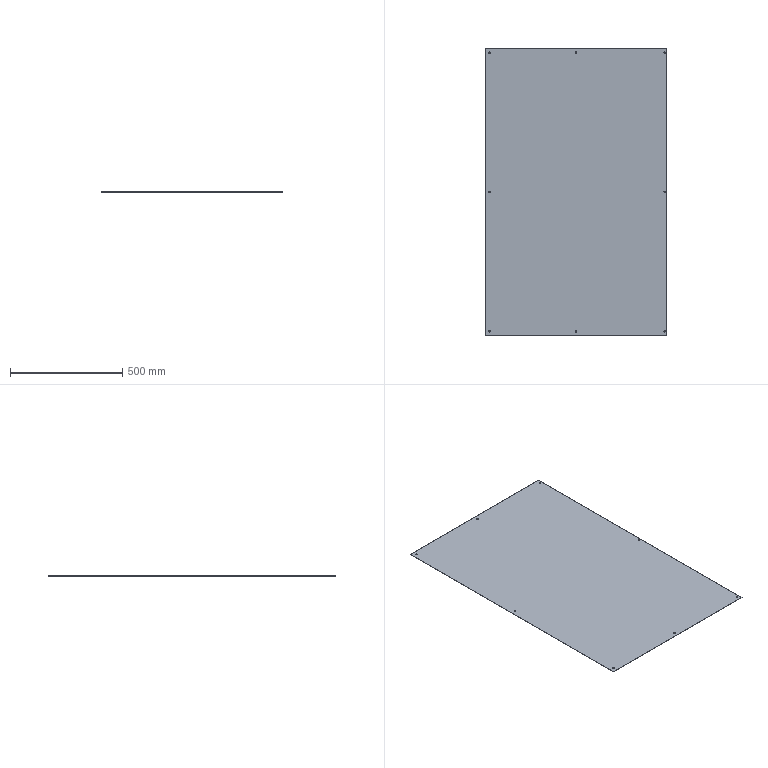Part | SolidWorks | features FlatPattern 1, HoleWzd 1, SMBaseFlange 1, SheetMetal 1 | 1 solid | 22 faces | box 810 x 1280 x 1.2 mm | volume 1243832 mm3 | cylinder 16 | plane 6 | commonest cylinder face diameters 6.6 x16
STEP:
#1=CARTESIAN_POINT('',(-388.3,620.,-1.2));
#2=VERTEX_POINT('',#1);
#3=CARTESIAN_POINT('',(-381.7,620.,-1.2));
#4=VERTEX_POINT('',#3);
#5=CARTESIAN_POINT('',(-385.,620.,-1.2));
#6=DIRECTION('',(0.,0.,1.));
#7=DIRECTION('',(1.,0.,0.));
#8=AXIS2_PLACEMENT_3D('',#5,#6,#7);
#9=CIRCLE('',#8,3.3);
#10=EDGE_CURVE('',#2,#4,#9,.T.);
#11=ORIENTED_EDGE('',*,*,#10,.F.);
#12=CARTESIAN_POINT('',(-388.3,620.,0.));
#13=VERTEX_POINT('',#12);
#14=CARTESIAN_POINT('',(-388.3,620.,0.));
#15=DIRECTION('',(0.,0.,1.));
#16=VECTOR('',#15,1000.);
#17=LINE('',#14,#16);
#18=EDGE_CURVE('',#2,#13,#17,.T.);
#19=ORIENTED_EDGE('',*,*,#18,.T.);
#20=CARTESIAN_POINT('',(-381.7,620.,0.));
#21=VERTEX_POINT('',#20);
#22=CARTESIAN_POINT('',(-385.,620.,0.));
#23=DIRECTION('',(0.,0.,1.));
#24=DIRECTION('',(1.,0.,0.));
#25=AXIS2_PLACEMENT_3D('',#22,#23,#24);
#26=CIRCLE('',#25,3.3);
#27=EDGE_CURVE('',#13,#21,#26,.T.);
#28=ORIENTED_EDGE('',*,*,#27,.T.);
#29=CARTESIAN_POINT('',(-381.7,620.,0.));
#30=DIRECTION('',(0.,0.,1.));
#31=VECTOR('',#30,1000.);
#32=LINE('',#29,#31);
#33=EDGE_CURVE('',#4,#21,#32,.T.);
#34=ORIENTED_EDGE('',*,*,#33,.F.);
#35=EDGE_LOOP('',(#11,#19,#28,#34));
#36=FACE_OUTER_BOUND('',#35,.T.);
#37=CARTESIAN_POINT('',(-385.,620.,0.));
#38=DIRECTION('',(0.,0.,1.));
#39=DIRECTION('',(1.,0.,0.));
#40=AXIS2_PLACEMENT_3D('',#37,#38,#39);
#41=CYLINDRICAL_SURFACE('',#40,3.3);
#42=ADVANCED_FACE('',(#36),#41,.F.);
#43=CARTESIAN_POINT('',(-3.3,620.,-1.2));
#44=VERTEX_POINT('',#43);
#45=CARTESIAN_POINT('',(3.3,620.,-1.2));
#46=VERTEX_POINT('',#45);
#47=CARTESIAN_POINT('',(0.,620.,-1.2));
#48=DIRECTION('',(0.,0.,1.));
#49=DIRECTION('',(1.,0.,0.));
#50=AXIS2_PLACEMENT_3D('',#47,#48,#49);
#51=CIRCLE('',#50,3.3);
#52=EDGE_CURVE('',#44,#46,#51,.T.);
#53=ORIENTED_EDGE('',*,*,#52,.F.);
#54=CARTESIAN_POINT('',(-3.3,620.,0.));
#55=VERTEX_POINT('',#54);
#56=CARTESIAN_POINT('',(-3.3,620.,0.));
#57=DIRECTION('',(0.,0.,1.));
#58=VECTOR('',#57,1000.);
#59=LINE('',#56,#58);
#60=EDGE_CURVE('',#44,#55,#59,.T.);
#61=ORIENTED_EDGE('',*,*,#60,.T.);
#62=CARTESIAN_POINT('',(3.3,620.,0.));
#63=VERTEX_POINT('',#62);
#64=CARTESIAN_POINT('',(0.,620.,0.));
#65=DIRECTION('',(0.,0.,1.));
#66=DIRECTION('',(1.,0.,0.));
#67=AXIS2_PLACEMENT_3D('',#64,#65,#66);
#68=CIRCLE('',#67,3.3);
#69=EDGE_CURVE('',#55,#63,#68,.T.);
#70=ORIENTED_EDGE('',*,*,#69,.T.);
#71=CARTESIAN_POINT('',(3.3,620.,0.));
#72=DIRECTION('',(0.,0.,1.));
#73=VECTOR('',#72,1000.);
#74=LINE('',#71,#73);
#75=EDGE_CURVE('',#46,#63,#74,.T.);
#76=ORIENTED_EDGE('',*,*,#75,.F.);
#77=EDGE_LOOP('',(#53,#61,#70,#76));
#78=FACE_OUTER_BOUND('',#77,.T.);
#79=CARTESIAN_POINT('',(0.,620.,0.));
#80=DIRECTION('',(0.,0.,1.));
#81=DIRECTION('',(1.,0.,0.));
#82=AXIS2_PLACEMENT_3D('',#79,#80,#81);
#83=CYLINDRICAL_SURFACE('',#82,3.3);
#84=ADVANCED_FACE('',(#78),#83,.F.);
#85=CARTESIAN_POINT('',(391.7,620.,-1.2));
#86=VERTEX_POINT('',#85);
#87=CARTESIAN_POINT('',(398.3,620.,-1.2));
#88=VERTEX_POINT('',#87);
#89=CARTESIAN_POINT('',(395.,620.,-1.2));
#90=DIRECTION('',(0.,0.,1.));
#91=DIRECTION('',(1.,0.,0.));
#92=AXIS2_PLACEMENT_3D('',#89,#90,#91);
#93=CIRCLE('',#92,3.3);
#94=EDGE_CURVE('',#86,#88,#93,.T.);
#95=ORIENTED_EDGE('',*,*,#94,.F.);
#96=CARTESIAN_POINT('',(391.7,620.,0.));
#97=VERTEX_POINT('',#96);
#98=CARTESIAN_POINT('',(391.7,620.,0.));
#99=DIRECTION('',(0.,0.,1.));
#100=VECTOR('',#99,1000.);
#101=LINE('',#98,#100);
#102=EDGE_CURVE('',#86,#97,#101,.T.);
#103=ORIENTED_EDGE('',*,*,#102,.T.);
#104=CARTESIAN_POINT('',(398.3,620.,0.));
#105=VERTEX_POINT('',#104);
#106=CARTESIAN_POINT('',(395.,620.,0.));
#107=DIRECTION('',(0.,0.,1.));
#108=DIRECTION('',(1.,0.,0.));
#109=AXIS2_PLACEMENT_3D('',#106,#107,#108);
#110=CIRCLE('',#109,3.3);
#111=EDGE_CURVE('',#97,#105,#110,.T.);
#112=ORIENTED_EDGE('',*,*,#111,.T.);
#113=CARTESIAN_POINT('',(398.3,620.,0.));
#114=DIRECTION('',(0.,0.,1.));
#115=VECTOR('',#114,1000.);
#116=LINE('',#113,#115);
#117=EDGE_CURVE('',#88,#105,#116,.T.);
#118=ORIENTED_EDGE('',*,*,#117,.F.);
#119=EDGE_LOOP('',(#95,#103,#112,#118));
#120=FACE_OUTER_BOUND('',#119,.T.);
#121=CARTESIAN_POINT('',(395.,620.,0.));
#122=DIRECTION('',(0.,0.,1.));
#123=DIRECTION('',(1.,0.,0.));
#124=AXIS2_PLACEMENT_3D('',#121,#122,#123);
#125=CYLINDRICAL_SURFACE('',#124,3.3);
#126=ADVANCED_FACE('',(#120),#125,.F.);
#127=CARTESIAN_POINT('',(391.7,0.,-1.2));
#128=VERTEX_POINT('',#127);
#129=CARTESIAN_POINT('',(398.3,0.,-1.2));
#130=VERTEX_POINT('',#129);
#131=CARTESIAN_POINT('',(395.,0.,-1.2));
#132=DIRECTION('',(0.,0.,1.));
#133=DIRECTION('',(1.,0.,0.));
#134=AXIS2_PLACEMENT_3D('',#131,#132,#133);
#135=CIRCLE('',#134,3.3);
#136=EDGE_CURVE('',#128,#130,#135,.T.);
#137=ORIENTED_EDGE('',*,*,#136,.F.);
#138=CARTESIAN_POINT('',(391.7,0.,0.));
#139=VERTEX_POINT('',#138);
#140=CARTESIAN_POINT('',(391.7,0.,0.));
#141=DIRECTION('',(0.,0.,1.));
#142=VECTOR('',#141,1000.);
#143=LINE('',#140,#142);
#144=EDGE_CURVE('',#128,#139,#143,.T.);
#145=ORIENTED_EDGE('',*,*,#144,.T.);
#146=CARTESIAN_POINT('',(398.3,0.,0.));
#147=VERTEX_POINT('',#146);
#148=CARTESIAN_POINT('',(395.,0.,0.));
#149=DIRECTION('',(0.,0.,1.));
#150=DIRECTION('',(1.,0.,0.));
#151=AXIS2_PLACEMENT_3D('',#148,#149,#150);
#152=CIRCLE('',#151,3.3);
#153=EDGE_CURVE('',#139,#147,#152,.T.);
#154=ORIENTED_EDGE('',*,*,#153,.T.);
#155=CARTESIAN_POINT('',(398.3,0.,0.));
#156=DIRECTION('',(0.,0.,1.));
#157=VECTOR('',#156,1000.);
#158=LINE('',#155,#157);
#159=EDGE_CURVE('',#130,#147,#158,.T.);
#160=ORIENTED_EDGE('',*,*,#159,.F.);
#161=EDGE_LOOP('',(#137,#145,#154,#160));
#162=FACE_OUTER_BOUND('',#161,.T.);
#163=CARTESIAN_POINT('',(395.,0.,0.));
#164=DIRECTION('',(0.,0.,1.));
#165=DIRECTION('',(1.,0.,0.));
#166=AXIS2_PLACEMENT_3D('',#163,#164,#165);
#167=CYLINDRICAL_SURFACE('',#166,3.3);
#168=ADVANCED_FACE('',(#162),#167,.F.);
#169=CARTESIAN_POINT('',(391.7,-620.,-1.2));
#170=VERTEX_POINT('',#169);
#171=CARTESIAN_POINT('',(398.3,-620.,-1.2));
#172=VERTEX_POINT('',#171);
#173=CARTESIAN_POINT('',(395.,-620.,-1.2));
#174=DIRECTION('',(0.,0.,1.));
#175=DIRECTION('',(1.,0.,0.));
#176=AXIS2_PLACEMENT_3D('',#173,#174,#175);
#177=CIRCLE('',#176,3.3);
#178=EDGE_CURVE('',#170,#172,#177,.T.);
#179=ORIENTED_EDGE('',*,*,#178,.F.);
#180=CARTESIAN_POINT('',(391.7,-620.,0.));
#181=VERTEX_POINT('',#180);
#182=CARTESIAN_POINT('',(391.7,-620.,0.));
#183=DIRECTION('',(0.,0.,1.));
#184=VECTOR('',#183,1000.);
#185=LINE('',#182,#184);
#186=EDGE_CURVE('',#170,#181,#185,.T.);
#187=ORIENTED_EDGE('',*,*,#186,.T.);
#188=CARTESIAN_POINT('',(398.3,-620.,0.));
#189=VERTEX_POINT('',#188);
#190=CARTESIAN_POINT('',(395.,-620.,0.));
#191=DIRECTION('',(0.,0.,1.));
#192=DIRECTION('',(1.,0.,0.));
#193=AXIS2_PLACEMENT_3D('',#190,#191,#192);
#194=CIRCLE('',#193,3.3);
#195=EDGE_CURVE('',#181,#189,#194,.T.);
#196=ORIENTED_EDGE('',*,*,#195,.T.);
#197=CARTESIAN_POINT('',(398.3,-620.,0.));
#198=DIRECTION('',(0.,0.,1.));
#199=VECTOR('',#198,1000.);
#200=LINE('',#197,#199);
#201=EDGE_CURVE('',#172,#189,#200,.T.);
#202=ORIENTED_EDGE('',*,*,#201,.F.);
#203=EDGE_LOOP('',(#179,#187,#196,#202));
#204=FACE_OUTER_BOUND('',#203,.T.);
#205=CARTESIAN_POINT('',(395.,-620.,0.));
#206=DIRECTION('',(0.,0.,1.));
#207=DIRECTION('',(1.,0.,0.));
#208=AXIS2_PLACEMENT_3D('',#205,#206,#207);
#209=CYLINDRICAL_SURFACE('',#208,3.3);
#210=ADVANCED_FACE('',(#204),#209,.F.);
#211=CARTESIAN_POINT('',(-3.3,-620.,-1.2));
#212=VERTEX_POINT('',#211);
#213=CARTESIAN_POINT('',(3.3,-620.,-1.2));
#214=VERTEX_POINT('',#213);
#215=CARTESIAN_POINT('',(0.,-620.,-1.2));
#216=DIRECTION('',(0.,0.,1.));
#217=DIRECTION('',(1.,0.,0.));
#218=AXIS2_PLACEMENT_3D('',#215,#216,#217);
#219=CIRCLE('',#218,3.3);
#220=EDGE_CURVE('',#212,#214,#219,.T.);
#221=ORIENTED_EDGE('',*,*,#220,.F.);
#222=CARTESIAN_POINT('',(-3.3,-620.,0.));
#223=VERTEX_POINT('',#222);
#224=CARTESIAN_POINT('',(-3.3,-620.,0.));
#225=DIRECTION('',(0.,0.,1.));
#226=VECTOR('',#225,1000.);
#227=LINE('',#224,#226);
#228=EDGE_CURVE('',#212,#223,#227,.T.);
#229=ORIENTED_EDGE('',*,*,#228,.T.);
#230=CARTESIAN_POINT('',(3.3,-620.,0.));
#231=VERTEX_POINT('',#230);
#232=CARTESIAN_POINT('',(0.,-620.,0.));
#233=DIRECTION('',(0.,0.,1.));
#234=DIRECTION('',(1.,0.,0.));
#235=AXIS2_PLACEMENT_3D('',#232,#233,#234);
#236=CIRCLE('',#235,3.3);
#237=EDGE_CURVE('',#223,#231,#236,.T.);
#238=ORIENTED_EDGE('',*,*,#237,.T.);
#239=CARTESIAN_POINT('',(3.3,-620.,0.));
#240=DIRECTION('',(0.,0.,1.));
#241=VECTOR('',#240,1000.);
#242=LINE('',#239,#241);
#243=EDGE_CURVE('',#214,#231,#242,.T.);
#244=ORIENTED_EDGE('',*,*,#243,.F.);
#245=EDGE_LOOP('',(#221,#229,#238,#244));
#246=FACE_OUTER_BOUND('',#245,.T.);
#247=CARTESIAN_POINT('',(0.,-620.,0.));
#248=DIRECTION('',(0.,0.,1.));
#249=DIRECTION('',(1.,0.,0.));
#250=AXIS2_PLACEMENT_3D('',#247,#248,#249);
#251=CYLINDRICAL_SURFACE('',#250,3.3);
#252=ADVANCED_FACE('',(#246),#251,.F.);
#253=CARTESIAN_POINT('',(-388.3,-620.,-1.2));
#254=VERTEX_POINT('',#253);
#255=CARTESIAN_POINT('',(-381.7,-620.,-1.2));
#256=VERTEX_POINT('',#255);
#257=CARTESIAN_POINT('',(-385.,-620.,-1.2));
#258=DIRECTION('',(0.,0.,1.));
#259=DIRECTION('',(1.,0.,0.));
#260=AXIS2_PLACEMENT_3D('',#257,#258,#259);
#261=CIRCLE('',#260,3.3);
#262=EDGE_CURVE('',#254,#256,#261,.T.);
#263=ORIENTED_EDGE('',*,*,#262,.F.);
#264=CARTESIAN_POINT('',(-388.3,-620.,0.));
#265=VERTEX_POINT('',#264);
#266=CARTESIAN_POINT('',(-388.3,-620.,0.));
#267=DIRECTION('',(0.,0.,1.));
#268=VECTOR('',#267,1000.);
#269=LINE('',#266,#268);
#270=EDGE_CURVE('',#254,#265,#269,.T.);
#271=ORIENTED_EDGE('',*,*,#270,.T.);
#272=CARTESIAN_POINT('',(-381.7,-620.,0.));
#273=VERTEX_POINT('',#272);
#274=CARTESIAN_POINT('',(-385.,-620.,0.));
#275=DIRECTION('',(0.,0.,1.));
#276=DIRECTION('',(1.,0.,0.));
#277=AXIS2_PLACEMENT_3D('',#274,#275,#276);
#278=CIRCLE('',#277,3.3);
#279=EDGE_CURVE('',#265,#273,#278,.T.);
#280=ORIENTED_EDGE('',*,*,#279,.T.);
#281=CARTESIAN_POINT('',(-381.7,-620.,0.));
#282=DIRECTION('',(0.,0.,1.));
#283=VECTOR('',#282,1000.);
#284=LINE('',#281,#283);
#285=EDGE_CURVE('',#256,#273,#284,.T.);
#286=ORIENTED_EDGE('',*,*,#285,.F.);
#287=EDGE_LOOP('',(#263,#271,#280,#286));
#288=FACE_OUTER_BOUND('',#287,.T.);
#289=CARTESIAN_POINT('',(-385.,-620.,0.));
#290=DIRECTION('',(0.,0.,1.));
#291=DIRECTION('',(1.,0.,0.));
#292=AXIS2_PLACEMENT_3D('',#289,#290,#291);
#293=CYLINDRICAL_SURFACE('',#292,3.3);
#294=ADVANCED_FACE('',(#288),#293,.F.);
#295=CARTESIAN_POINT('',(-388.3,0.,-1.2));
#296=VERTEX_POINT('',#295);
#297=CARTESIAN_POINT('',(-381.7,0.,-1.2));
#298=VERTEX_POINT('',#297);
#299=CARTESIAN_POINT('',(-385.,0.,-1.2));
#300=DIRECTION('',(0.,0.,1.));
#301=DIRECTION('',(1.,0.,0.));
#302=AXIS2_PLACEMENT_3D('',#299,#300,#301);
#303=CIRCLE('',#302,3.3);
#304=EDGE_CURVE('',#296,#298,#303,.T.);
#305=ORIENTED_EDGE('',*,*,#304,.F.);
#306=CARTESIAN_POINT('',(-388.3,0.,0.));
#307=VERTEX_POINT('',#306);
#308=CARTESIAN_POINT('',(-388.3,0.,0.));
#309=DIRECTION('',(0.,0.,1.));
#310=VECTOR('',#309,1000.);
#311=LINE('',#308,#310);
#312=EDGE_CURVE('',#296,#307,#311,.T.);
#313=ORIENTED_EDGE('',*,*,#312,.T.);
#314=CARTESIAN_POINT('',(-381.7,0.,0.));
#315=VERTEX_POINT('',#314);
#316=CARTESIAN_POINT('',(-385.,0.,0.));
#317=DIRECTION('',(0.,0.,1.));
#318=DIRECTION('',(1.,0.,0.));
#319=AXIS2_PLACEMENT_3D('',#316,#317,#318);
#320=CIRCLE('',#319,3.3);
#321=EDGE_CURVE('',#307,#315,#320,.T.);
#322=ORIENTED_EDGE('',*,*,#321,.T.);
#323=CARTESIAN_POINT('',(-381.7,0.,0.));
#324=DIRECTION('',(0.,0.,1.));
#325=VECTOR('',#324,1000.);
#326=LINE('',#323,#325);
#327=EDGE_CURVE('',#298,#315,#326,.T.);
#328=ORIENTED_EDGE('',*,*,#327,.F.);
#329=EDGE_LOOP('',(#305,#313,#322,#328));
#330=FACE_OUTER_BOUND('',#329,.T.);
#331=CARTESIAN_POINT('',(-385.,0.,0.));
#332=DIRECTION('',(0.,0.,1.));
#333=DIRECTION('',(1.,0.,0.));
#334=AXIS2_PLACEMENT_3D('',#331,#332,#333);
#335=CYLINDRICAL_SURFACE('',#334,3.3);
#336=ADVANCED_FACE('',(#330),#335,.F.);
#337=CARTESIAN_POINT('',(405.,-640.,0.));
#338=VERTEX_POINT('',#337);
#339=CARTESIAN_POINT('',(405.,640.,0.));
#340=VERTEX_POINT('',#339);
#341=CARTESIAN_POINT('',(405.,640.,0.));
#342=DIRECTION('',(0.,1.,0.));
#343=VECTOR('',#342,1000.);
#344=LINE('',#341,#343);
#345=EDGE_CURVE('',#338,#340,#344,.T.);
#346=ORIENTED_EDGE('',*,*,#345,.F.);
#347=CARTESIAN_POINT('',(405.,-640.,-1.2));
#348=VERTEX_POINT('',#347);
#349=CARTESIAN_POINT('',(405.,-640.,-1.2));
#350=DIRECTION('',(0.,0.,1.));
#351=VECTOR('',#350,1000.);
#352=LINE('',#349,#351);
#353=EDGE_CURVE('',#348,#338,#352,.T.);
#354=ORIENTED_EDGE('',*,*,#353,.F.);
#355=CARTESIAN_POINT('',(405.,640.,-1.2));
#356=VERTEX_POINT('',#355);
#357=CARTESIAN_POINT('',(405.,640.,-1.2));
#358=DIRECTION('',(0.,1.,0.));
#359=VECTOR('',#358,1000.);
#360=LINE('',#357,#359);
#361=EDGE_CURVE('',#348,#356,#360,.T.);
#362=ORIENTED_EDGE('',*,*,#361,.T.);
#363=CARTESIAN_POINT('',(405.,640.,-1.2));
#364=DIRECTION('',(0.,0.,1.));
#365=VECTOR('',#364,1000.);
#366=LINE('',#363,#365);
#367=EDGE_CURVE('',#356,#340,#366,.T.);
#368=ORIENTED_EDGE('',*,*,#367,.T.);
#369=EDGE_LOOP('',(#346,#354,#362,#368));
#370=FACE_OUTER_BOUND('',#369,.T.);
#371=CARTESIAN_POINT('',(405.,640.,-1.2));
#372=DIRECTION('',(1.,0.,0.));
#373=DIRECTION('',(0.,1.,0.));
#374=AXIS2_PLACEMENT_3D('',#371,#372,#373);
#375=PLANE('',#374);
#376=ADVANCED_FACE('',(#370),#375,.T.);
#377=CARTESIAN_POINT('',(-405.,-640.,0.));
#378=VERTEX_POINT('',#377);
#379=CARTESIAN_POINT('',(-405.,-640.,0.));
#380=DIRECTION('',(1.,0.,0.));
#381=VECTOR('',#380,1000.);
#382=LINE('',#379,#381);
#383=EDGE_CURVE('',#378,#338,#382,.T.);
#384=ORIENTED_EDGE('',*,*,#383,.F.);
#385=CARTESIAN_POINT('',(-405.,-640.,-1.2));
#386=VERTEX_POINT('',#385);
#387=CARTESIAN_POINT('',(-405.,-640.,-1.2));
#388=DIRECTION('',(0.,0.,1.));
#389=VECTOR('',#388,1000.);
#390=LINE('',#387,#389);
#391=EDGE_CURVE('',#386,#378,#390,.T.);
#392=ORIENTED_EDGE('',*,*,#391,.F.);
#393=CARTESIAN_POINT('',(-405.,-640.,-1.2));
#394=DIRECTION('',(1.,0.,0.));
#395=VECTOR('',#394,1000.);
#396=LINE('',#393,#395);
#397=EDGE_CURVE('',#386,#348,#396,.T.);
#398=ORIENTED_EDGE('',*,*,#397,.T.);
#399=ORIENTED_EDGE('',*,*,#353,.T.);
#400=EDGE_LOOP('',(#384,#392,#398,#399));
#401=FACE_OUTER_BOUND('',#400,.T.);
#402=CARTESIAN_POINT('',(-405.,-640.,-1.2));
#403=DIRECTION('',(0.,-1.,0.));
#404=DIRECTION('',(0.,0.,-1.));
#405=AXIS2_PLACEMENT_3D('',#402,#403,#404);
#406=PLANE('',#405);
#407=ADVANCED_FACE('',(#401),#406,.T.);
#408=CARTESIAN_POINT('',(-405.,640.,0.));
#409=VERTEX_POINT('',#408);
#410=CARTESIAN_POINT('',(-405.,640.,0.));
#411=DIRECTION('',(0.,-1.,0.));
#412=VECTOR('',#411,1000.);
#413=LINE('',#410,#412);
#414=EDGE_CURVE('',#409,#378,#413,.T.);
#415=ORIENTED_EDGE('',*,*,#414,.F.);
#416=CARTESIAN_POINT('',(-405.,640.,-1.2));
#417=VERTEX_POINT('',#416);
#418=CARTESIAN_POINT('',(-405.,640.,-1.2));
#419=DIRECTION('',(0.,0.,1.));
#420=VECTOR('',#419,1000.);
#421=LINE('',#418,#420);
#422=EDGE_CURVE('',#417,#409,#421,.T.);
#423=ORIENTED_EDGE('',*,*,#422,.F.);
#424=CARTESIAN_POINT('',(-405.,640.,-1.2));
#425=DIRECTION('',(0.,-1.,0.));
#426=VECTOR('',#425,1000.);
#427=LINE('',#424,#426);
#428=EDGE_CURVE('',#417,#386,#427,.T.);
#429=ORIENTED_EDGE('',*,*,#428,.T.);
#430=ORIENTED_EDGE('',*,*,#391,.T.);
#431=EDGE_LOOP('',(#415,#423,#429,#430));
#432=FACE_OUTER_BOUND('',#431,.T.);
#433=CARTESIAN_POINT('',(-405.,640.,-1.2));
#434=DIRECTION('',(-1.,0.,0.));
#435=DIRECTION('',(0.,-1.,0.));
#436=AXIS2_PLACEMENT_3D('',#433,#434,#435);
#437=PLANE('',#436);
#438=ADVANCED_FACE('',(#432),#437,.T.);
#439=CARTESIAN_POINT('',(-405.,640.,0.));
#440=DIRECTION('',(-1.,0.,0.));
#441=VECTOR('',#440,1000.);
#442=LINE('',#439,#441);
#443=EDGE_CURVE('',#340,#409,#442,.T.);
#444=ORIENTED_EDGE('',*,*,#443,.F.);
#445=ORIENTED_EDGE('',*,*,#367,.F.);
#446=CARTESIAN_POINT('',(-405.,640.,-1.2));
#447=DIRECTION('',(-1.,0.,0.));
#448=VECTOR('',#447,1000.);
#449=LINE('',#446,#448);
#450=EDGE_CURVE('',#356,#417,#449,.T.);
#451=ORIENTED_EDGE('',*,*,#450,.T.);
#452=ORIENTED_EDGE('',*,*,#422,.T.);
#453=EDGE_LOOP('',(#444,#445,#451,#452));
#454=FACE_OUTER_BOUND('',#453,.T.);
#455=CARTESIAN_POINT('',(-405.,640.,-1.2));
#456=DIRECTION('',(0.,1.,0.));
#457=DIRECTION('',(0.,0.,1.));
#458=AXIS2_PLACEMENT_3D('',#455,#456,#457);
#459=PLANE('',#458);
#460=ADVANCED_FACE('',(#454),#459,.T.);
#461=CARTESIAN_POINT('',(-385.,620.,-1.2));
#462=DIRECTION('',(0.,0.,1.));
#463=DIRECTION('',(1.,0.,0.));
#464=AXIS2_PLACEMENT_3D('',#461,#462,#463);
#465=CIRCLE('',#464,3.3);
#466=EDGE_CURVE('',#4,#2,#465,.T.);
#467=ORIENTED_EDGE('',*,*,#466,.T.);
#468=ORIENTED_EDGE('',*,*,#10,.T.);
#469=EDGE_LOOP('',(#467,#468));
#470=FACE_BOUND('',#469,.T.);
#471=CARTESIAN_POINT('',(0.,620.,-1.2));
#472=DIRECTION('',(0.,0.,1.));
#473=DIRECTION('',(1.,0.,0.));
#474=AXIS2_PLACEMENT_3D('',#471,#472,#473);
#475=CIRCLE('',#474,3.3);
#476=EDGE_CURVE('',#46,#44,#475,.T.);
#477=ORIENTED_EDGE('',*,*,#476,.T.);
#478=ORIENTED_EDGE('',*,*,#52,.T.);
#479=EDGE_LOOP('',(#477,#478));
#480=FACE_BOUND('',#479,.T.);
#481=CARTESIAN_POINT('',(395.,620.,-1.2));
#482=DIRECTION('',(0.,0.,1.));
#483=DIRECTION('',(1.,0.,0.));
#484=AXIS2_PLACEMENT_3D('',#481,#482,#483);
#485=CIRCLE('',#484,3.3);
#486=EDGE_CURVE('',#88,#86,#485,.T.);
#487=ORIENTED_EDGE('',*,*,#486,.T.);
#488=ORIENTED_EDGE('',*,*,#94,.T.);
#489=EDGE_LOOP('',(#487,#488));
#490=FACE_BOUND('',#489,.T.);
#491=CARTESIAN_POINT('',(395.,0.,-1.2));
#492=DIRECTION('',(0.,0.,1.));
#493=DIRECTION('',(1.,0.,0.));
#494=AXIS2_PLACEMENT_3D('',#491,#492,#493);
#495=CIRCLE('',#494,3.3);
#496=EDGE_CURVE('',#130,#128,#495,.T.);
#497=ORIENTED_EDGE('',*,*,#496,.T.);
#498=ORIENTED_EDGE('',*,*,#136,.T.);
#499=EDGE_LOOP('',(#497,#498));
#500=FACE_BOUND('',#499,.T.);
#501=CARTESIAN_POINT('',(395.,-620.,-1.2));
#502=DIRECTION('',(0.,0.,1.));
#503=DIRECTION('',(1.,0.,0.));
#504=AXIS2_PLACEMENT_3D('',#501,#502,#503);
#505=CIRCLE('',#504,3.3);
#506=EDGE_CURVE('',#172,#170,#505,.T.);
#507=ORIENTED_EDGE('',*,*,#506,.T.);
#508=ORIENTED_EDGE('',*,*,#178,.T.);
#509=EDGE_LOOP('',(#507,#508));
#510=FACE_BOUND('',#509,.T.);
#511=CARTESIAN_POINT('',(0.,-620.,-1.2));
#512=DIRECTION('',(0.,0.,1.));
#513=DIRECTION('',(1.,0.,0.));
#514=AXIS2_PLACEMENT_3D('',#511,#512,#513);
#515=CIRCLE('',#514,3.3);
#516=EDGE_CURVE('',#214,#212,#515,.T.);
#517=ORIENTED_EDGE('',*,*,#516,.T.);
#518=ORIENTED_EDGE('',*,*,#220,.T.);
#519=EDGE_LOOP('',(#517,#518));
#520=FACE_BOUND('',#519,.T.);
#521=CARTESIAN_POINT('',(-385.,-620.,-1.2));
#522=DIRECTION('',(0.,0.,1.));
#523=DIRECTION('',(1.,0.,0.));
#524=AXIS2_PLACEMENT_3D('',#521,#522,#523);
#525=CIRCLE('',#524,3.3);
#526=EDGE_CURVE('',#256,#254,#525,.T.);
#527=ORIENTED_EDGE('',*,*,#526,.T.);
#528=ORIENTED_EDGE('',*,*,#262,.T.);
#529=EDGE_LOOP('',(#527,#528));
#530=FACE_BOUND('',#529,.T.);
#531=CARTESIAN_POINT('',(-385.,0.,-1.2));
#532=DIRECTION('',(0.,0.,1.));
#533=DIRECTION('',(1.,0.,0.));
#534=AXIS2_PLACEMENT_3D('',#531,#532,#533);
#535=CIRCLE('',#534,3.3);
#536=EDGE_CURVE('',#298,#296,#535,.T.);
#537=ORIENTED_EDGE('',*,*,#536,.T.);
#538=ORIENTED_EDGE('',*,*,#304,.T.);
#539=EDGE_LOOP('',(#537,#538));
#540=FACE_BOUND('',#539,.T.);
#541=ORIENTED_EDGE('',*,*,#361,.F.);
#542=ORIENTED_EDGE('',*,*,#397,.F.);
#543=ORIENTED_EDGE('',*,*,#428,.F.);
#544=ORIENTED_EDGE('',*,*,#450,.F.);
#545=EDGE_LOOP('',(#541,#542,#543,#544));
#546=FACE_OUTER_BOUND('',#545,.T.);
#547=CARTESIAN_POINT('',(0.,0.,-1.2));
#548=DIRECTION('',(0.,0.,1.));
#549=DIRECTION('',(1.,0.,0.));
#550=AXIS2_PLACEMENT_3D('',#547,#548,#549);
#551=PLANE('',#550);
#552=ADVANCED_FACE('',(#470,#480,#490,#500,#510,#520,#530,#540,#546),#551,.F.);
#553=CARTESIAN_POINT('',(-385.,620.,0.));
#554=DIRECTION('',(0.,0.,1.));
#555=DIRECTION('',(1.,0.,0.));
#556=AXIS2_PLACEMENT_3D('',#553,#554,#555);
#557=CIRCLE('',#556,3.3);
#558=EDGE_CURVE('',#21,#13,#557,.T.);
#559=ORIENTED_EDGE('',*,*,#558,.F.);
#560=ORIENTED_EDGE('',*,*,#27,.F.);
#561=EDGE_LOOP('',(#559,#560));
#562=FACE_BOUND('',#561,.T.);
#563=CARTESIAN_POINT('',(0.,620.,0.));
#564=DIRECTION('',(0.,0.,1.));
#565=DIRECTION('',(1.,0.,0.));
#566=AXIS2_PLACEMENT_3D('',#563,#564,#565);
#567=CIRCLE('',#566,3.3);
#568=EDGE_CURVE('',#63,#55,#567,.T.);
#569=ORIENTED_EDGE('',*,*,#568,.F.);
#570=ORIENTED_EDGE('',*,*,#69,.F.);
#571=EDGE_LOOP('',(#569,#570));
#572=FACE_BOUND('',#571,.T.);
#573=CARTESIAN_POINT('',(395.,620.,0.));
#574=DIRECTION('',(0.,0.,1.));
#575=DIRECTION('',(1.,0.,0.));
#576=AXIS2_PLACEMENT_3D('',#573,#574,#575);
#577=CIRCLE('',#576,3.3);
#578=EDGE_CURVE('',#105,#97,#577,.T.);
#579=ORIENTED_EDGE('',*,*,#578,.F.);
#580=ORIENTED_EDGE('',*,*,#111,.F.);
#581=EDGE_LOOP('',(#579,#580));
#582=FACE_BOUND('',#581,.T.);
#583=CARTESIAN_POINT('',(395.,0.,0.));
#584=DIRECTION('',(0.,0.,1.));
#585=DIRECTION('',(1.,0.,0.));
#586=AXIS2_PLACEMENT_3D('',#583,#584,#585);
#587=CIRCLE('',#586,3.3);
#588=EDGE_CURVE('',#147,#139,#587,.T.);
#589=ORIENTED_EDGE('',*,*,#588,.F.);
#590=ORIENTED_EDGE('',*,*,#153,.F.);
#591=EDGE_LOOP('',(#589,#590));
#592=FACE_BOUND('',#591,.T.);
#593=CARTESIAN_POINT('',(395.,-620.,0.));
#594=DIRECTION('',(0.,0.,1.));
#595=DIRECTION('',(1.,0.,0.));
#596=AXIS2_PLACEMENT_3D('',#593,#594,#595);
#597=CIRCLE('',#596,3.3);
#598=EDGE_CURVE('',#189,#181,#597,.T.);
#599=ORIENTED_EDGE('',*,*,#598,.F.);
#600=ORIENTED_EDGE('',*,*,#195,.F.);
#601=EDGE_LOOP('',(#599,#600));
#602=FACE_BOUND('',#601,.T.);
#603=CARTESIAN_POINT('',(0.,-620.,0.));
#604=DIRECTION('',(0.,0.,1.));
#605=DIRECTION('',(1.,0.,0.));
#606=AXIS2_PLACEMENT_3D('',#603,#604,#605);
#607=CIRCLE('',#606,3.3);
#608=EDGE_CURVE('',#231,#223,#607,.T.);
#609=ORIENTED_EDGE('',*,*,#608,.F.);
#610=ORIENTED_EDGE('',*,*,#237,.F.);
#611=EDGE_LOOP('',(#609,#610));
#612=FACE_BOUND('',#611,.T.);
#613=CARTESIAN_POINT('',(-385.,-620.,0.));
#614=DIRECTION('',(0.,0.,1.));
#615=DIRECTION('',(1.,0.,0.));
#616=AXIS2_PLACEMENT_3D('',#613,#614,#615);
#617=CIRCLE('',#616,3.3);
#618=EDGE_CURVE('',#273,#265,#617,.T.);
#619=ORIENTED_EDGE('',*,*,#618,.F.);
#620=ORIENTED_EDGE('',*,*,#279,.F.);
#621=EDGE_LOOP('',(#619,#620));
#622=FACE_BOUND('',#621,.T.);
#623=CARTESIAN_POINT('',(-385.,0.,0.));
#624=DIRECTION('',(0.,0.,1.));
#625=DIRECTION('',(1.,0.,0.));
#626=AXIS2_PLACEMENT_3D('',#623,#624,#625);
#627=CIRCLE('',#626,3.3);
#628=EDGE_CURVE('',#315,#307,#627,.T.);
#629=ORIENTED_EDGE('',*,*,#628,.F.);
#630=ORIENTED_EDGE('',*,*,#321,.F.);
#631=EDGE_LOOP('',(#629,#630));
#632=FACE_BOUND('',#631,.T.);
#633=ORIENTED_EDGE('',*,*,#345,.T.);
#634=ORIENTED_EDGE('',*,*,#443,.T.);
#635=ORIENTED_EDGE('',*,*,#414,.T.);
#636=ORIENTED_EDGE('',*,*,#383,.T.);
#637=EDGE_LOOP('',(#633,#634,#635,#636));
#638=FACE_OUTER_BOUND('',#637,.T.);
#639=CARTESIAN_POINT('',(0.,0.,0.));
#640=DIRECTION('',(0.,0.,1.));
#641=DIRECTION('',(1.,0.,0.));
#642=AXIS2_PLACEMENT_3D('',#639,#640,#641);
#643=PLANE('',#642);
#644=ADVANCED_FACE('',(#562,#572,#582,#592,#602,#612,#622,#632,#638),#643,.T.);
#645=ORIENTED_EDGE('',*,*,#312,.F.);
#646=ORIENTED_EDGE('',*,*,#536,.F.);
#647=ORIENTED_EDGE('',*,*,#327,.T.);
#648=ORIENTED_EDGE('',*,*,#628,.T.);
#649=EDGE_LOOP('',(#645,#646,#647,#648));
#650=FACE_OUTER_BOUND('',#649,.T.);
#651=CARTESIAN_POINT('',(-385.,0.,0.));
#652=DIRECTION('',(0.,0.,1.));
#653=DIRECTION('',(1.,0.,0.));
#654=AXIS2_PLACEMENT_3D('',#651,#652,#653);
#655=CYLINDRICAL_SURFACE('',#654,3.3);
#656=ADVANCED_FACE('',(#650),#655,.F.);
#657=ORIENTED_EDGE('',*,*,#270,.F.);
#658=ORIENTED_EDGE('',*,*,#526,.F.);
#659=ORIENTED_EDGE('',*,*,#285,.T.);
#660=ORIENTED_EDGE('',*,*,#618,.T.);
#661=EDGE_LOOP('',(#657,#658,#659,#660));
#662=FACE_OUTER_BOUND('',#661,.T.);
#663=CARTESIAN_POINT('',(-385.,-620.,0.));
#664=DIRECTION('',(0.,0.,1.));
#665=DIRECTION('',(1.,0.,0.));
#666=AXIS2_PLACEMENT_3D('',#663,#664,#665);
#667=CYLINDRICAL_SURFACE('',#666,3.3);
#668=ADVANCED_FACE('',(#662),#667,.F.);
#669=ORIENTED_EDGE('',*,*,#228,.F.);
#670=ORIENTED_EDGE('',*,*,#516,.F.);
#671=ORIENTED_EDGE('',*,*,#243,.T.);
#672=ORIENTED_EDGE('',*,*,#608,.T.);
#673=EDGE_LOOP('',(#669,#670,#671,#672));
#674=FACE_OUTER_BOUND('',#673,.T.);
#675=CARTESIAN_POINT('',(0.,-620.,0.));
#676=DIRECTION('',(0.,0.,1.));
#677=DIRECTION('',(1.,0.,0.));
#678=AXIS2_PLACEMENT_3D('',#675,#676,#677);
#679=CYLINDRICAL_SURFACE('',#678,3.3);
#680=ADVANCED_FACE('',(#674),#679,.F.);
#681=ORIENTED_EDGE('',*,*,#186,.F.);
#682=ORIENTED_EDGE('',*,*,#506,.F.);
#683=ORIENTED_EDGE('',*,*,#201,.T.);
#684=ORIENTED_EDGE('',*,*,#598,.T.);
#685=EDGE_LOOP('',(#681,#682,#683,#684));
#686=FACE_OUTER_BOUND('',#685,.T.);
#687=CARTESIAN_POINT('',(395.,-620.,0.));
#688=DIRECTION('',(0.,0.,1.));
#689=DIRECTION('',(1.,0.,0.));
#690=AXIS2_PLACEMENT_3D('',#687,#688,#689);
#691=CYLINDRICAL_SURFACE('',#690,3.3);
#692=ADVANCED_FACE('',(#686),#691,.F.);
#693=ORIENTED_EDGE('',*,*,#144,.F.);
#694=ORIENTED_EDGE('',*,*,#496,.F.);
#695=ORIENTED_EDGE('',*,*,#159,.T.);
#696=ORIENTED_EDGE('',*,*,#588,.T.);
#697=EDGE_LOOP('',(#693,#694,#695,#696));
#698=FACE_OUTER_BOUND('',#697,.T.);
#699=CARTESIAN_POINT('',(395.,0.,0.));
#700=DIRECTION('',(0.,0.,1.));
#701=DIRECTION('',(1.,0.,0.));
#702=AXIS2_PLACEMENT_3D('',#699,#700,#701);
#703=CYLINDRICAL_SURFACE('',#702,3.3);
#704=ADVANCED_FACE('',(#698),#703,.F.);
#705=ORIENTED_EDGE('',*,*,#102,.F.);
#706=ORIENTED_EDGE('',*,*,#486,.F.);
#707=ORIENTED_EDGE('',*,*,#117,.T.);
#708=ORIENTED_EDGE('',*,*,#578,.T.);
#709=EDGE_LOOP('',(#705,#706,#707,#708));
#710=FACE_OUTER_BOUND('',#709,.T.);
#711=CARTESIAN_POINT('',(395.,620.,0.));
#712=DIRECTION('',(0.,0.,1.));
#713=DIRECTION('',(1.,0.,0.));
#714=AXIS2_PLACEMENT_3D('',#711,#712,#713);
#715=CYLINDRICAL_SURFACE('',#714,3.3);
#716=ADVANCED_FACE('',(#710),#715,.F.);
#717=ORIENTED_EDGE('',*,*,#60,.F.);
#718=ORIENTED_EDGE('',*,*,#476,.F.);
#719=ORIENTED_EDGE('',*,*,#75,.T.);
#720=ORIENTED_EDGE('',*,*,#568,.T.);
#721=EDGE_LOOP('',(#717,#718,#719,#720));
#722=FACE_OUTER_BOUND('',#721,.T.);
#723=CARTESIAN_POINT('',(0.,620.,0.));
#724=DIRECTION('',(0.,0.,1.));
#725=DIRECTION('',(1.,0.,0.));
#726=AXIS2_PLACEMENT_3D('',#723,#724,#725);
#727=CYLINDRICAL_SURFACE('',#726,3.3);
#728=ADVANCED_FACE('',(#722),#727,.F.);
#729=ORIENTED_EDGE('',*,*,#18,.F.);
#730=ORIENTED_EDGE('',*,*,#466,.F.);
#731=ORIENTED_EDGE('',*,*,#33,.T.);
#732=ORIENTED_EDGE('',*,*,#558,.T.);
#733=EDGE_LOOP('',(#729,#730,#731,#732));
#734=FACE_OUTER_BOUND('',#733,.T.);
#735=CARTESIAN_POINT('',(-385.,620.,0.));
#736=DIRECTION('',(0.,0.,1.));
#737=DIRECTION('',(1.,0.,0.));
#738=AXIS2_PLACEMENT_3D('',#735,#736,#737);
#739=CYLINDRICAL_SURFACE('',#738,3.3);
#740=ADVANCED_FACE('',(#734),#739,.F.);
#741=CLOSED_SHELL('',(#42,#84,#126,#168,#210,#252,#294,#336,#376,#407,#438,#460,#552,#644,#656,#668,#680,#692,#704,#716,#728,#740));
#742=MANIFOLD_SOLID_BREP('',#741);
#743=CARTESIAN_POINT('',(0.,0.,0.));
#744=DIRECTION('',(0.,0.,1.));
#745=DIRECTION('',(1.,0.,0.));
#746=AXIS2_PLACEMENT_3D('',#743,#744,#745);
#747=(LENGTH_UNIT()NAMED_UNIT(*)SI_UNIT(.MILLI.,.METRE.));
#748=UNCERTAINTY_MEASURE_WITH_UNIT(LENGTH_MEASURE(0.00001),#747,'','');
#749=(NAMED_UNIT(*)PLANE_ANGLE_UNIT()SI_UNIT($,.RADIAN.));
#750=(NAMED_UNIT(*)SI_UNIT($,.STERADIAN.)SOLID_ANGLE_UNIT());
#751=(GEOMETRIC_REPRESENTATION_CONTEXT(3)GLOBAL_UNCERTAINTY_ASSIGNED_CONTEXT((#748))GLOBAL_UNIT_ASSIGNED_CONTEXT((#747,#749,#750))REPRESENTATION_CONTEXT('',''));
#752=ADVANCED_BREP_SHAPE_REPRESENTATION('',(#742,#746),#751);